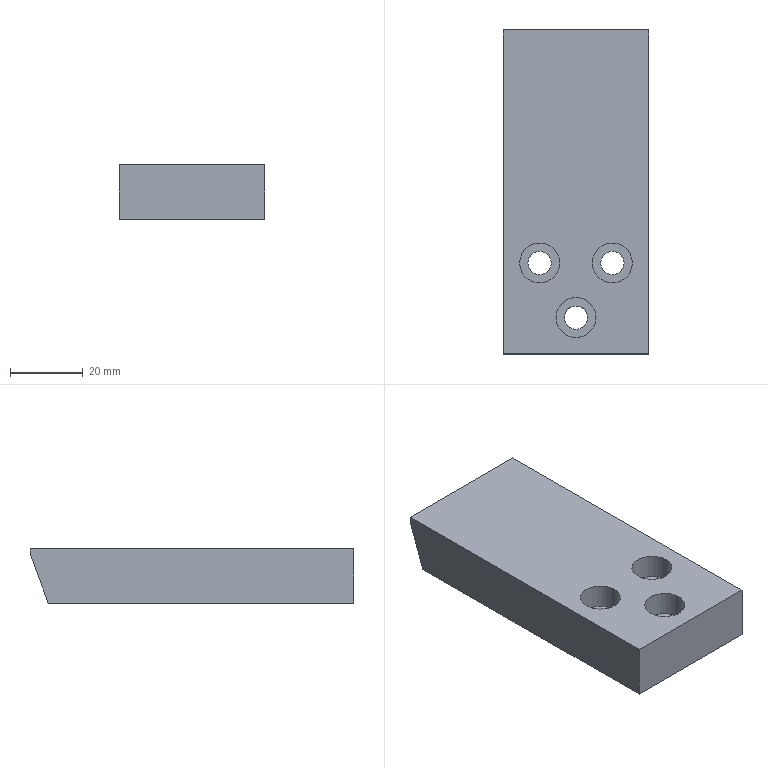Part | SolidWorks | features BaseBody 1 | 1 solid | 22 faces | box 40 x 89 x 15 mm | volume 49296 mm3 | cylinder 12 | plane 10 | commonest cylinder face diameters 6.4 x6 11 x6
STEP:
#1=CARTESIAN_POINT('',(4.5,25.,8.2));
#2=VERTEX_POINT('',#1);
#3=CARTESIAN_POINT('',(15.5,25.,8.2));
#4=VERTEX_POINT('',#3);
#5=CARTESIAN_POINT('',(10.,25.,8.2));
#6=DIRECTION('',(0.,0.,1.));
#7=DIRECTION('',(1.,0.,0.));
#8=AXIS2_PLACEMENT_3D('',#5,#6,#7);
#9=CIRCLE('',#8,5.5);
#10=EDGE_CURVE('',#2,#4,#9,.T.);
#11=ORIENTED_EDGE('',*,*,#10,.F.);
#12=CARTESIAN_POINT('',(4.5,25.,15.));
#13=VERTEX_POINT('',#12);
#14=CARTESIAN_POINT('',(4.5,25.,15.));
#15=DIRECTION('',(0.,0.,1.));
#16=VECTOR('',#15,1000.);
#17=LINE('',#14,#16);
#18=EDGE_CURVE('',#2,#13,#17,.T.);
#19=ORIENTED_EDGE('',*,*,#18,.T.);
#20=CARTESIAN_POINT('',(15.5,25.,15.));
#21=VERTEX_POINT('',#20);
#22=CARTESIAN_POINT('',(10.,25.,15.));
#23=DIRECTION('',(0.,0.,1.));
#24=DIRECTION('',(1.,0.,0.));
#25=AXIS2_PLACEMENT_3D('',#22,#23,#24);
#26=CIRCLE('',#25,5.5);
#27=EDGE_CURVE('',#13,#21,#26,.T.);
#28=ORIENTED_EDGE('',*,*,#27,.T.);
#29=CARTESIAN_POINT('',(15.5,25.,15.));
#30=DIRECTION('',(0.,0.,1.));
#31=VECTOR('',#30,1000.);
#32=LINE('',#29,#31);
#33=EDGE_CURVE('',#4,#21,#32,.T.);
#34=ORIENTED_EDGE('',*,*,#33,.F.);
#35=EDGE_LOOP('',(#11,#19,#28,#34));
#36=FACE_OUTER_BOUND('',#35,.T.);
#37=CARTESIAN_POINT('',(10.,25.,15.));
#38=DIRECTION('',(0.,0.,1.));
#39=DIRECTION('',(1.,0.,0.));
#40=AXIS2_PLACEMENT_3D('',#37,#38,#39);
#41=CYLINDRICAL_SURFACE('',#40,5.5);
#42=ADVANCED_FACE('',(#36),#41,.F.);
#43=CARTESIAN_POINT('',(6.8,25.,0.));
#44=VERTEX_POINT('',#43);
#45=CARTESIAN_POINT('',(13.2,25.,0.));
#46=VERTEX_POINT('',#45);
#47=CARTESIAN_POINT('',(10.,25.,0.));
#48=DIRECTION('',(0.,0.,1.));
#49=DIRECTION('',(1.,0.,0.));
#50=AXIS2_PLACEMENT_3D('',#47,#48,#49);
#51=CIRCLE('',#50,3.2);
#52=EDGE_CURVE('',#44,#46,#51,.T.);
#53=ORIENTED_EDGE('',*,*,#52,.F.);
#54=CARTESIAN_POINT('',(6.8,25.,8.2));
#55=VERTEX_POINT('',#54);
#56=CARTESIAN_POINT('',(6.8,25.,15.));
#57=DIRECTION('',(0.,0.,1.));
#58=VECTOR('',#57,1000.);
#59=LINE('',#56,#58);
#60=EDGE_CURVE('',#44,#55,#59,.T.);
#61=ORIENTED_EDGE('',*,*,#60,.T.);
#62=CARTESIAN_POINT('',(13.2,25.,8.2));
#63=VERTEX_POINT('',#62);
#64=CARTESIAN_POINT('',(10.,25.,8.2));
#65=DIRECTION('',(0.,0.,1.));
#66=DIRECTION('',(1.,0.,0.));
#67=AXIS2_PLACEMENT_3D('',#64,#65,#66);
#68=CIRCLE('',#67,3.2);
#69=EDGE_CURVE('',#55,#63,#68,.T.);
#70=ORIENTED_EDGE('',*,*,#69,.T.);
#71=CARTESIAN_POINT('',(13.2,25.,15.));
#72=DIRECTION('',(0.,0.,1.));
#73=VECTOR('',#72,1000.);
#74=LINE('',#71,#73);
#75=EDGE_CURVE('',#46,#63,#74,.T.);
#76=ORIENTED_EDGE('',*,*,#75,.F.);
#77=EDGE_LOOP('',(#53,#61,#70,#76));
#78=FACE_OUTER_BOUND('',#77,.T.);
#79=CARTESIAN_POINT('',(10.,25.,15.));
#80=DIRECTION('',(0.,0.,1.));
#81=DIRECTION('',(1.,0.,0.));
#82=AXIS2_PLACEMENT_3D('',#79,#80,#81);
#83=CYLINDRICAL_SURFACE('',#82,3.2);
#84=ADVANCED_FACE('',(#78),#83,.F.);
#85=CARTESIAN_POINT('',(24.5,25.,8.2));
#86=VERTEX_POINT('',#85);
#87=CARTESIAN_POINT('',(35.5,25.,8.2));
#88=VERTEX_POINT('',#87);
#89=CARTESIAN_POINT('',(30.,25.,8.2));
#90=DIRECTION('',(0.,0.,1.));
#91=DIRECTION('',(1.,0.,0.));
#92=AXIS2_PLACEMENT_3D('',#89,#90,#91);
#93=CIRCLE('',#92,5.5);
#94=EDGE_CURVE('',#86,#88,#93,.T.);
#95=ORIENTED_EDGE('',*,*,#94,.F.);
#96=CARTESIAN_POINT('',(24.5,25.,15.));
#97=VERTEX_POINT('',#96);
#98=CARTESIAN_POINT('',(24.5,25.,15.));
#99=DIRECTION('',(0.,0.,1.));
#100=VECTOR('',#99,1000.);
#101=LINE('',#98,#100);
#102=EDGE_CURVE('',#86,#97,#101,.T.);
#103=ORIENTED_EDGE('',*,*,#102,.T.);
#104=CARTESIAN_POINT('',(35.5,25.,15.));
#105=VERTEX_POINT('',#104);
#106=CARTESIAN_POINT('',(30.,25.,15.));
#107=DIRECTION('',(0.,0.,1.));
#108=DIRECTION('',(1.,0.,0.));
#109=AXIS2_PLACEMENT_3D('',#106,#107,#108);
#110=CIRCLE('',#109,5.5);
#111=EDGE_CURVE('',#97,#105,#110,.T.);
#112=ORIENTED_EDGE('',*,*,#111,.T.);
#113=CARTESIAN_POINT('',(35.5,25.,15.));
#114=DIRECTION('',(0.,0.,1.));
#115=VECTOR('',#114,1000.);
#116=LINE('',#113,#115);
#117=EDGE_CURVE('',#88,#105,#116,.T.);
#118=ORIENTED_EDGE('',*,*,#117,.F.);
#119=EDGE_LOOP('',(#95,#103,#112,#118));
#120=FACE_OUTER_BOUND('',#119,.T.);
#121=CARTESIAN_POINT('',(30.,25.,15.));
#122=DIRECTION('',(0.,0.,1.));
#123=DIRECTION('',(1.,0.,0.));
#124=AXIS2_PLACEMENT_3D('',#121,#122,#123);
#125=CYLINDRICAL_SURFACE('',#124,5.5);
#126=ADVANCED_FACE('',(#120),#125,.F.);
#127=CARTESIAN_POINT('',(26.8,25.,0.));
#128=VERTEX_POINT('',#127);
#129=CARTESIAN_POINT('',(33.2,25.,0.));
#130=VERTEX_POINT('',#129);
#131=CARTESIAN_POINT('',(30.,25.,0.));
#132=DIRECTION('',(0.,0.,1.));
#133=DIRECTION('',(1.,0.,0.));
#134=AXIS2_PLACEMENT_3D('',#131,#132,#133);
#135=CIRCLE('',#134,3.2);
#136=EDGE_CURVE('',#128,#130,#135,.T.);
#137=ORIENTED_EDGE('',*,*,#136,.F.);
#138=CARTESIAN_POINT('',(26.8,25.,8.2));
#139=VERTEX_POINT('',#138);
#140=CARTESIAN_POINT('',(26.8,25.,15.));
#141=DIRECTION('',(0.,0.,1.));
#142=VECTOR('',#141,1000.);
#143=LINE('',#140,#142);
#144=EDGE_CURVE('',#128,#139,#143,.T.);
#145=ORIENTED_EDGE('',*,*,#144,.T.);
#146=CARTESIAN_POINT('',(33.2,25.,8.2));
#147=VERTEX_POINT('',#146);
#148=CARTESIAN_POINT('',(30.,25.,8.2));
#149=DIRECTION('',(0.,0.,1.));
#150=DIRECTION('',(1.,0.,0.));
#151=AXIS2_PLACEMENT_3D('',#148,#149,#150);
#152=CIRCLE('',#151,3.2);
#153=EDGE_CURVE('',#139,#147,#152,.T.);
#154=ORIENTED_EDGE('',*,*,#153,.T.);
#155=CARTESIAN_POINT('',(33.2,25.,15.));
#156=DIRECTION('',(0.,0.,1.));
#157=VECTOR('',#156,1000.);
#158=LINE('',#155,#157);
#159=EDGE_CURVE('',#130,#147,#158,.T.);
#160=ORIENTED_EDGE('',*,*,#159,.F.);
#161=EDGE_LOOP('',(#137,#145,#154,#160));
#162=FACE_OUTER_BOUND('',#161,.T.);
#163=CARTESIAN_POINT('',(30.,25.,15.));
#164=DIRECTION('',(0.,0.,1.));
#165=DIRECTION('',(1.,0.,0.));
#166=AXIS2_PLACEMENT_3D('',#163,#164,#165);
#167=CYLINDRICAL_SURFACE('',#166,3.2);
#168=ADVANCED_FACE('',(#162),#167,.F.);
#169=CARTESIAN_POINT('',(14.5,10.,8.2));
#170=VERTEX_POINT('',#169);
#171=CARTESIAN_POINT('',(25.5,10.,8.2));
#172=VERTEX_POINT('',#171);
#173=CARTESIAN_POINT('',(20.,10.,8.2));
#174=DIRECTION('',(0.,0.,1.));
#175=DIRECTION('',(1.,0.,0.));
#176=AXIS2_PLACEMENT_3D('',#173,#174,#175);
#177=CIRCLE('',#176,5.5);
#178=EDGE_CURVE('',#170,#172,#177,.T.);
#179=ORIENTED_EDGE('',*,*,#178,.F.);
#180=CARTESIAN_POINT('',(14.5,10.,15.));
#181=VERTEX_POINT('',#180);
#182=CARTESIAN_POINT('',(14.5,10.,15.));
#183=DIRECTION('',(0.,0.,1.));
#184=VECTOR('',#183,1000.);
#185=LINE('',#182,#184);
#186=EDGE_CURVE('',#170,#181,#185,.T.);
#187=ORIENTED_EDGE('',*,*,#186,.T.);
#188=CARTESIAN_POINT('',(25.5,10.,15.));
#189=VERTEX_POINT('',#188);
#190=CARTESIAN_POINT('',(20.,10.,15.));
#191=DIRECTION('',(0.,0.,1.));
#192=DIRECTION('',(1.,0.,0.));
#193=AXIS2_PLACEMENT_3D('',#190,#191,#192);
#194=CIRCLE('',#193,5.5);
#195=EDGE_CURVE('',#181,#189,#194,.T.);
#196=ORIENTED_EDGE('',*,*,#195,.T.);
#197=CARTESIAN_POINT('',(25.5,10.,15.));
#198=DIRECTION('',(0.,0.,1.));
#199=VECTOR('',#198,1000.);
#200=LINE('',#197,#199);
#201=EDGE_CURVE('',#172,#189,#200,.T.);
#202=ORIENTED_EDGE('',*,*,#201,.F.);
#203=EDGE_LOOP('',(#179,#187,#196,#202));
#204=FACE_OUTER_BOUND('',#203,.T.);
#205=CARTESIAN_POINT('',(20.,10.,15.));
#206=DIRECTION('',(0.,0.,1.));
#207=DIRECTION('',(1.,0.,0.));
#208=AXIS2_PLACEMENT_3D('',#205,#206,#207);
#209=CYLINDRICAL_SURFACE('',#208,5.5);
#210=ADVANCED_FACE('',(#204),#209,.F.);
#211=CARTESIAN_POINT('',(16.8,10.,0.));
#212=VERTEX_POINT('',#211);
#213=CARTESIAN_POINT('',(23.2,10.,0.));
#214=VERTEX_POINT('',#213);
#215=CARTESIAN_POINT('',(20.,10.,0.));
#216=DIRECTION('',(0.,0.,1.));
#217=DIRECTION('',(1.,0.,0.));
#218=AXIS2_PLACEMENT_3D('',#215,#216,#217);
#219=CIRCLE('',#218,3.2);
#220=EDGE_CURVE('',#212,#214,#219,.T.);
#221=ORIENTED_EDGE('',*,*,#220,.F.);
#222=CARTESIAN_POINT('',(16.8,10.,8.2));
#223=VERTEX_POINT('',#222);
#224=CARTESIAN_POINT('',(16.8,10.,15.));
#225=DIRECTION('',(0.,0.,1.));
#226=VECTOR('',#225,1000.);
#227=LINE('',#224,#226);
#228=EDGE_CURVE('',#212,#223,#227,.T.);
#229=ORIENTED_EDGE('',*,*,#228,.T.);
#230=CARTESIAN_POINT('',(23.2,10.,8.2));
#231=VERTEX_POINT('',#230);
#232=CARTESIAN_POINT('',(20.,10.,8.2));
#233=DIRECTION('',(0.,0.,1.));
#234=DIRECTION('',(1.,0.,0.));
#235=AXIS2_PLACEMENT_3D('',#232,#233,#234);
#236=CIRCLE('',#235,3.2);
#237=EDGE_CURVE('',#223,#231,#236,.T.);
#238=ORIENTED_EDGE('',*,*,#237,.T.);
#239=CARTESIAN_POINT('',(23.2,10.,15.));
#240=DIRECTION('',(0.,0.,1.));
#241=VECTOR('',#240,1000.);
#242=LINE('',#239,#241);
#243=EDGE_CURVE('',#214,#231,#242,.T.);
#244=ORIENTED_EDGE('',*,*,#243,.F.);
#245=EDGE_LOOP('',(#221,#229,#238,#244));
#246=FACE_OUTER_BOUND('',#245,.T.);
#247=CARTESIAN_POINT('',(20.,10.,15.));
#248=DIRECTION('',(0.,0.,1.));
#249=DIRECTION('',(1.,0.,0.));
#250=AXIS2_PLACEMENT_3D('',#247,#248,#249);
#251=CYLINDRICAL_SURFACE('',#250,3.2);
#252=ADVANCED_FACE('',(#246),#251,.F.);
#253=CARTESIAN_POINT('',(40.,84.,0.));
#254=VERTEX_POINT('',#253);
#255=CARTESIAN_POINT('',(40.,89.,13.737));
#256=VERTEX_POINT('',#255);
#257=CARTESIAN_POINT('',(40.,89.,13.737));
#258=DIRECTION('',(0.,0.342,0.9397));
#259=VECTOR('',#258,1000.);
#260=LINE('',#257,#259);
#261=EDGE_CURVE('',#254,#256,#260,.T.);
#262=ORIENTED_EDGE('',*,*,#261,.F.);
#263=CARTESIAN_POINT('',(0.,84.,0.));
#264=VERTEX_POINT('',#263);
#265=CARTESIAN_POINT('',(40.,84.,0.));
#266=DIRECTION('',(1.,0.,0.));
#267=VECTOR('',#266,1000.);
#268=LINE('',#265,#267);
#269=EDGE_CURVE('',#264,#254,#268,.T.);
#270=ORIENTED_EDGE('',*,*,#269,.F.);
#271=CARTESIAN_POINT('',(0.,89.,13.737));
#272=VERTEX_POINT('',#271);
#273=CARTESIAN_POINT('',(0.,89.,13.737));
#274=DIRECTION('',(0.,-0.342,-0.9397));
#275=VECTOR('',#274,1000.);
#276=LINE('',#273,#275);
#277=EDGE_CURVE('',#272,#264,#276,.T.);
#278=ORIENTED_EDGE('',*,*,#277,.F.);
#279=CARTESIAN_POINT('',(0.,89.,13.737));
#280=DIRECTION('',(-1.,0.,0.));
#281=VECTOR('',#280,1000.);
#282=LINE('',#279,#281);
#283=EDGE_CURVE('',#256,#272,#282,.T.);
#284=ORIENTED_EDGE('',*,*,#283,.F.);
#285=EDGE_LOOP('',(#262,#270,#278,#284));
#286=FACE_OUTER_BOUND('',#285,.T.);
#287=CARTESIAN_POINT('',(0.,89.,13.737));
#288=DIRECTION('',(0.,0.9397,-0.342));
#289=DIRECTION('',(-1.,0.,0.));
#290=AXIS2_PLACEMENT_3D('',#287,#288,#289);
#291=PLANE('',#290);
#292=ADVANCED_FACE('',(#286),#291,.T.);
#293=CARTESIAN_POINT('',(10.,25.,8.2));
#294=DIRECTION('',(0.,0.,1.));
#295=DIRECTION('',(1.,0.,0.));
#296=AXIS2_PLACEMENT_3D('',#293,#294,#295);
#297=CIRCLE('',#296,3.2);
#298=EDGE_CURVE('',#63,#55,#297,.T.);
#299=ORIENTED_EDGE('',*,*,#298,.F.);
#300=ORIENTED_EDGE('',*,*,#69,.F.);
#301=EDGE_LOOP('',(#299,#300));
#302=FACE_BOUND('',#301,.T.);
#303=CARTESIAN_POINT('',(10.,25.,8.2));
#304=DIRECTION('',(0.,0.,1.));
#305=DIRECTION('',(1.,0.,0.));
#306=AXIS2_PLACEMENT_3D('',#303,#304,#305);
#307=CIRCLE('',#306,5.5);
#308=EDGE_CURVE('',#4,#2,#307,.T.);
#309=ORIENTED_EDGE('',*,*,#308,.T.);
#310=ORIENTED_EDGE('',*,*,#10,.T.);
#311=EDGE_LOOP('',(#309,#310));
#312=FACE_OUTER_BOUND('',#311,.T.);
#313=CARTESIAN_POINT('',(13.2,25.,8.2));
#314=DIRECTION('',(0.,0.,-1.));
#315=DIRECTION('',(0.,-1.,0.));
#316=AXIS2_PLACEMENT_3D('',#313,#314,#315);
#317=PLANE('',#316);
#318=ADVANCED_FACE('',(#302,#312),#317,.F.);
#319=CARTESIAN_POINT('',(30.,25.,8.2));
#320=DIRECTION('',(0.,0.,1.));
#321=DIRECTION('',(1.,0.,0.));
#322=AXIS2_PLACEMENT_3D('',#319,#320,#321);
#323=CIRCLE('',#322,3.2);
#324=EDGE_CURVE('',#147,#139,#323,.T.);
#325=ORIENTED_EDGE('',*,*,#324,.F.);
#326=ORIENTED_EDGE('',*,*,#153,.F.);
#327=EDGE_LOOP('',(#325,#326));
#328=FACE_BOUND('',#327,.T.);
#329=CARTESIAN_POINT('',(30.,25.,8.2));
#330=DIRECTION('',(0.,0.,1.));
#331=DIRECTION('',(1.,0.,0.));
#332=AXIS2_PLACEMENT_3D('',#329,#330,#331);
#333=CIRCLE('',#332,5.5);
#334=EDGE_CURVE('',#88,#86,#333,.T.);
#335=ORIENTED_EDGE('',*,*,#334,.T.);
#336=ORIENTED_EDGE('',*,*,#94,.T.);
#337=EDGE_LOOP('',(#335,#336));
#338=FACE_OUTER_BOUND('',#337,.T.);
#339=CARTESIAN_POINT('',(33.2,25.,8.2));
#340=DIRECTION('',(0.,0.,-1.));
#341=DIRECTION('',(0.,-1.,0.));
#342=AXIS2_PLACEMENT_3D('',#339,#340,#341);
#343=PLANE('',#342);
#344=ADVANCED_FACE('',(#328,#338),#343,.F.);
#345=CARTESIAN_POINT('',(20.,10.,8.2));
#346=DIRECTION('',(0.,0.,1.));
#347=DIRECTION('',(1.,0.,0.));
#348=AXIS2_PLACEMENT_3D('',#345,#346,#347);
#349=CIRCLE('',#348,3.2);
#350=EDGE_CURVE('',#231,#223,#349,.T.);
#351=ORIENTED_EDGE('',*,*,#350,.F.);
#352=ORIENTED_EDGE('',*,*,#237,.F.);
#353=EDGE_LOOP('',(#351,#352));
#354=FACE_BOUND('',#353,.T.);
#355=CARTESIAN_POINT('',(20.,10.,8.2));
#356=DIRECTION('',(0.,0.,1.));
#357=DIRECTION('',(1.,0.,0.));
#358=AXIS2_PLACEMENT_3D('',#355,#356,#357);
#359=CIRCLE('',#358,5.5);
#360=EDGE_CURVE('',#172,#170,#359,.T.);
#361=ORIENTED_EDGE('',*,*,#360,.T.);
#362=ORIENTED_EDGE('',*,*,#178,.T.);
#363=EDGE_LOOP('',(#361,#362));
#364=FACE_OUTER_BOUND('',#363,.T.);
#365=CARTESIAN_POINT('',(23.2,10.,8.2));
#366=DIRECTION('',(0.,0.,-1.));
#367=DIRECTION('',(0.,-1.,0.));
#368=AXIS2_PLACEMENT_3D('',#365,#366,#367);
#369=PLANE('',#368);
#370=ADVANCED_FACE('',(#354,#364),#369,.F.);
#371=CARTESIAN_POINT('',(20.,10.,0.));
#372=DIRECTION('',(0.,0.,1.));
#373=DIRECTION('',(1.,0.,0.));
#374=AXIS2_PLACEMENT_3D('',#371,#372,#373);
#375=CIRCLE('',#374,3.2);
#376=EDGE_CURVE('',#214,#212,#375,.T.);
#377=ORIENTED_EDGE('',*,*,#376,.T.);
#378=ORIENTED_EDGE('',*,*,#220,.T.);
#379=EDGE_LOOP('',(#377,#378));
#380=FACE_BOUND('',#379,.T.);
#381=CARTESIAN_POINT('',(30.,25.,0.));
#382=DIRECTION('',(0.,0.,1.));
#383=DIRECTION('',(1.,0.,0.));
#384=AXIS2_PLACEMENT_3D('',#381,#382,#383);
#385=CIRCLE('',#384,3.2);
#386=EDGE_CURVE('',#130,#128,#385,.T.);
#387=ORIENTED_EDGE('',*,*,#386,.T.);
#388=ORIENTED_EDGE('',*,*,#136,.T.);
#389=EDGE_LOOP('',(#387,#388));
#390=FACE_BOUND('',#389,.T.);
#391=CARTESIAN_POINT('',(10.,25.,0.));
#392=DIRECTION('',(0.,0.,1.));
#393=DIRECTION('',(1.,0.,0.));
#394=AXIS2_PLACEMENT_3D('',#391,#392,#393);
#395=CIRCLE('',#394,3.2);
#396=EDGE_CURVE('',#46,#44,#395,.T.);
#397=ORIENTED_EDGE('',*,*,#396,.T.);
#398=ORIENTED_EDGE('',*,*,#52,.T.);
#399=EDGE_LOOP('',(#397,#398));
#400=FACE_BOUND('',#399,.T.);
#401=CARTESIAN_POINT('',(0.,0.,0.));
#402=VERTEX_POINT('',#401);
#403=CARTESIAN_POINT('',(0.,0.,0.));
#404=DIRECTION('',(0.,-1.,0.));
#405=VECTOR('',#404,1000.);
#406=LINE('',#403,#405);
#407=EDGE_CURVE('',#264,#402,#406,.T.);
#408=ORIENTED_EDGE('',*,*,#407,.F.);
#409=ORIENTED_EDGE('',*,*,#269,.T.);
#410=CARTESIAN_POINT('',(40.,0.,0.));
#411=VERTEX_POINT('',#410);
#412=CARTESIAN_POINT('',(40.,0.,0.));
#413=DIRECTION('',(0.,1.,0.));
#414=VECTOR('',#413,1000.);
#415=LINE('',#412,#414);
#416=EDGE_CURVE('',#411,#254,#415,.T.);
#417=ORIENTED_EDGE('',*,*,#416,.F.);
#418=CARTESIAN_POINT('',(0.,0.,0.));
#419=DIRECTION('',(1.,0.,0.));
#420=VECTOR('',#419,1000.);
#421=LINE('',#418,#420);
#422=EDGE_CURVE('',#402,#411,#421,.T.);
#423=ORIENTED_EDGE('',*,*,#422,.F.);
#424=EDGE_LOOP('',(#408,#409,#417,#423));
#425=FACE_OUTER_BOUND('',#424,.T.);
#426=CARTESIAN_POINT('',(0.,0.,0.));
#427=DIRECTION('',(0.,0.,-1.));
#428=DIRECTION('',(0.,-1.,0.));
#429=AXIS2_PLACEMENT_3D('',#426,#427,#428);
#430=PLANE('',#429);
#431=ADVANCED_FACE('',(#380,#390,#400,#425),#430,.T.);
#432=CARTESIAN_POINT('',(20.,10.,15.));
#433=DIRECTION('',(0.,0.,1.));
#434=DIRECTION('',(1.,0.,0.));
#435=AXIS2_PLACEMENT_3D('',#432,#433,#434);
#436=CIRCLE('',#435,5.5);
#437=EDGE_CURVE('',#189,#181,#436,.T.);
#438=ORIENTED_EDGE('',*,*,#437,.F.);
#439=ORIENTED_EDGE('',*,*,#195,.F.);
#440=EDGE_LOOP('',(#438,#439));
#441=FACE_BOUND('',#440,.T.);
#442=CARTESIAN_POINT('',(30.,25.,15.));
#443=DIRECTION('',(0.,0.,1.));
#444=DIRECTION('',(1.,0.,0.));
#445=AXIS2_PLACEMENT_3D('',#442,#443,#444);
#446=CIRCLE('',#445,5.5);
#447=EDGE_CURVE('',#105,#97,#446,.T.);
#448=ORIENTED_EDGE('',*,*,#447,.F.);
#449=ORIENTED_EDGE('',*,*,#111,.F.);
#450=EDGE_LOOP('',(#448,#449));
#451=FACE_BOUND('',#450,.T.);
#452=CARTESIAN_POINT('',(10.,25.,15.));
#453=DIRECTION('',(0.,0.,1.));
#454=DIRECTION('',(1.,0.,0.));
#455=AXIS2_PLACEMENT_3D('',#452,#453,#454);
#456=CIRCLE('',#455,5.5);
#457=EDGE_CURVE('',#21,#13,#456,.T.);
#458=ORIENTED_EDGE('',*,*,#457,.F.);
#459=ORIENTED_EDGE('',*,*,#27,.F.);
#460=EDGE_LOOP('',(#458,#459));
#461=FACE_BOUND('',#460,.T.);
#462=CARTESIAN_POINT('',(0.,89.,15.));
#463=VERTEX_POINT('',#462);
#464=CARTESIAN_POINT('',(0.,0.,15.));
#465=VERTEX_POINT('',#464);
#466=CARTESIAN_POINT('',(0.,0.,15.));
#467=DIRECTION('',(0.,-1.,0.));
#468=VECTOR('',#467,1000.);
#469=LINE('',#466,#468);
#470=EDGE_CURVE('',#463,#465,#469,.T.);
#471=ORIENTED_EDGE('',*,*,#470,.T.);
#472=CARTESIAN_POINT('',(40.,0.,15.));
#473=VERTEX_POINT('',#472);
#474=CARTESIAN_POINT('',(0.,0.,15.));
#475=DIRECTION('',(1.,0.,0.));
#476=VECTOR('',#475,1000.);
#477=LINE('',#474,#476);
#478=EDGE_CURVE('',#465,#473,#477,.T.);
#479=ORIENTED_EDGE('',*,*,#478,.T.);
#480=CARTESIAN_POINT('',(40.,89.,15.));
#481=VERTEX_POINT('',#480);
#482=CARTESIAN_POINT('',(40.,0.,15.));
#483=DIRECTION('',(0.,1.,0.));
#484=VECTOR('',#483,1000.);
#485=LINE('',#482,#484);
#486=EDGE_CURVE('',#473,#481,#485,.T.);
#487=ORIENTED_EDGE('',*,*,#486,.T.);
#488=CARTESIAN_POINT('',(0.,89.,15.));
#489=DIRECTION('',(-1.,0.,0.));
#490=VECTOR('',#489,1000.);
#491=LINE('',#488,#490);
#492=EDGE_CURVE('',#481,#463,#491,.T.);
#493=ORIENTED_EDGE('',*,*,#492,.T.);
#494=EDGE_LOOP('',(#471,#479,#487,#493));
#495=FACE_OUTER_BOUND('',#494,.T.);
#496=CARTESIAN_POINT('',(0.,0.,15.));
#497=DIRECTION('',(0.,0.,-1.));
#498=DIRECTION('',(0.,-1.,0.));
#499=AXIS2_PLACEMENT_3D('',#496,#497,#498);
#500=PLANE('',#499);
#501=ADVANCED_FACE('',(#441,#451,#461,#495),#500,.F.);
#502=CARTESIAN_POINT('',(40.,89.,15.));
#503=DIRECTION('',(0.,0.,-1.));
#504=VECTOR('',#503,1000.);
#505=LINE('',#502,#504);
#506=EDGE_CURVE('',#481,#256,#505,.T.);
#507=ORIENTED_EDGE('',*,*,#506,.T.);
#508=ORIENTED_EDGE('',*,*,#283,.T.);
#509=CARTESIAN_POINT('',(0.,89.,15.));
#510=DIRECTION('',(0.,0.,-1.));
#511=VECTOR('',#510,1000.);
#512=LINE('',#509,#511);
#513=EDGE_CURVE('',#463,#272,#512,.T.);
#514=ORIENTED_EDGE('',*,*,#513,.F.);
#515=ORIENTED_EDGE('',*,*,#492,.F.);
#516=EDGE_LOOP('',(#507,#508,#514,#515));
#517=FACE_OUTER_BOUND('',#516,.T.);
#518=CARTESIAN_POINT('',(0.,89.,15.));
#519=DIRECTION('',(0.,-1.,0.));
#520=DIRECTION('',(0.,0.,-1.));
#521=AXIS2_PLACEMENT_3D('',#518,#519,#520);
#522=PLANE('',#521);
#523=ADVANCED_FACE('',(#517),#522,.F.);
#524=ORIENTED_EDGE('',*,*,#416,.T.);
#525=ORIENTED_EDGE('',*,*,#261,.T.);
#526=ORIENTED_EDGE('',*,*,#506,.F.);
#527=ORIENTED_EDGE('',*,*,#486,.F.);
#528=CARTESIAN_POINT('',(40.,0.,15.));
#529=DIRECTION('',(0.,0.,-1.));
#530=VECTOR('',#529,1000.);
#531=LINE('',#528,#530);
#532=EDGE_CURVE('',#473,#411,#531,.T.);
#533=ORIENTED_EDGE('',*,*,#532,.T.);
#534=EDGE_LOOP('',(#524,#525,#526,#527,#533));
#535=FACE_OUTER_BOUND('',#534,.T.);
#536=CARTESIAN_POINT('',(40.,0.,15.));
#537=DIRECTION('',(-1.,0.,0.));
#538=DIRECTION('',(0.,0.,1.));
#539=AXIS2_PLACEMENT_3D('',#536,#537,#538);
#540=PLANE('',#539);
#541=ADVANCED_FACE('',(#535),#540,.F.);
#542=ORIENTED_EDGE('',*,*,#422,.T.);
#543=ORIENTED_EDGE('',*,*,#532,.F.);
#544=ORIENTED_EDGE('',*,*,#478,.F.);
#545=CARTESIAN_POINT('',(0.,0.,15.));
#546=DIRECTION('',(0.,0.,-1.));
#547=VECTOR('',#546,1000.);
#548=LINE('',#545,#547);
#549=EDGE_CURVE('',#465,#402,#548,.T.);
#550=ORIENTED_EDGE('',*,*,#549,.T.);
#551=EDGE_LOOP('',(#542,#543,#544,#550));
#552=FACE_OUTER_BOUND('',#551,.T.);
#553=CARTESIAN_POINT('',(0.,0.,15.));
#554=DIRECTION('',(0.,1.,0.));
#555=DIRECTION('',(1.,0.,0.));
#556=AXIS2_PLACEMENT_3D('',#553,#554,#555);
#557=PLANE('',#556);
#558=ADVANCED_FACE('',(#552),#557,.F.);
#559=ORIENTED_EDGE('',*,*,#513,.T.);
#560=ORIENTED_EDGE('',*,*,#277,.T.);
#561=ORIENTED_EDGE('',*,*,#407,.T.);
#562=ORIENTED_EDGE('',*,*,#549,.F.);
#563=ORIENTED_EDGE('',*,*,#470,.F.);
#564=EDGE_LOOP('',(#559,#560,#561,#562,#563));
#565=FACE_OUTER_BOUND('',#564,.T.);
#566=CARTESIAN_POINT('',(0.,0.,15.));
#567=DIRECTION('',(1.,0.,0.));
#568=DIRECTION('',(0.,1.,0.));
#569=AXIS2_PLACEMENT_3D('',#566,#567,#568);
#570=PLANE('',#569);
#571=ADVANCED_FACE('',(#565),#570,.F.);
#572=ORIENTED_EDGE('',*,*,#228,.F.);
#573=ORIENTED_EDGE('',*,*,#376,.F.);
#574=ORIENTED_EDGE('',*,*,#243,.T.);
#575=ORIENTED_EDGE('',*,*,#350,.T.);
#576=EDGE_LOOP('',(#572,#573,#574,#575));
#577=FACE_OUTER_BOUND('',#576,.T.);
#578=CARTESIAN_POINT('',(20.,10.,15.));
#579=DIRECTION('',(0.,0.,1.));
#580=DIRECTION('',(1.,0.,0.));
#581=AXIS2_PLACEMENT_3D('',#578,#579,#580);
#582=CYLINDRICAL_SURFACE('',#581,3.2);
#583=ADVANCED_FACE('',(#577),#582,.F.);
#584=ORIENTED_EDGE('',*,*,#186,.F.);
#585=ORIENTED_EDGE('',*,*,#360,.F.);
#586=ORIENTED_EDGE('',*,*,#201,.T.);
#587=ORIENTED_EDGE('',*,*,#437,.T.);
#588=EDGE_LOOP('',(#584,#585,#586,#587));
#589=FACE_OUTER_BOUND('',#588,.T.);
#590=CARTESIAN_POINT('',(20.,10.,15.));
#591=DIRECTION('',(0.,0.,1.));
#592=DIRECTION('',(1.,0.,0.));
#593=AXIS2_PLACEMENT_3D('',#590,#591,#592);
#594=CYLINDRICAL_SURFACE('',#593,5.5);
#595=ADVANCED_FACE('',(#589),#594,.F.);
#596=ORIENTED_EDGE('',*,*,#144,.F.);
#597=ORIENTED_EDGE('',*,*,#386,.F.);
#598=ORIENTED_EDGE('',*,*,#159,.T.);
#599=ORIENTED_EDGE('',*,*,#324,.T.);
#600=EDGE_LOOP('',(#596,#597,#598,#599));
#601=FACE_OUTER_BOUND('',#600,.T.);
#602=CARTESIAN_POINT('',(30.,25.,15.));
#603=DIRECTION('',(0.,0.,1.));
#604=DIRECTION('',(1.,0.,0.));
#605=AXIS2_PLACEMENT_3D('',#602,#603,#604);
#606=CYLINDRICAL_SURFACE('',#605,3.2);
#607=ADVANCED_FACE('',(#601),#606,.F.);
#608=ORIENTED_EDGE('',*,*,#102,.F.);
#609=ORIENTED_EDGE('',*,*,#334,.F.);
#610=ORIENTED_EDGE('',*,*,#117,.T.);
#611=ORIENTED_EDGE('',*,*,#447,.T.);
#612=EDGE_LOOP('',(#608,#609,#610,#611));
#613=FACE_OUTER_BOUND('',#612,.T.);
#614=CARTESIAN_POINT('',(30.,25.,15.));
#615=DIRECTION('',(0.,0.,1.));
#616=DIRECTION('',(1.,0.,0.));
#617=AXIS2_PLACEMENT_3D('',#614,#615,#616);
#618=CYLINDRICAL_SURFACE('',#617,5.5);
#619=ADVANCED_FACE('',(#613),#618,.F.);
#620=ORIENTED_EDGE('',*,*,#60,.F.);
#621=ORIENTED_EDGE('',*,*,#396,.F.);
#622=ORIENTED_EDGE('',*,*,#75,.T.);
#623=ORIENTED_EDGE('',*,*,#298,.T.);
#624=EDGE_LOOP('',(#620,#621,#622,#623));
#625=FACE_OUTER_BOUND('',#624,.T.);
#626=CARTESIAN_POINT('',(10.,25.,15.));
#627=DIRECTION('',(0.,0.,1.));
#628=DIRECTION('',(1.,0.,0.));
#629=AXIS2_PLACEMENT_3D('',#626,#627,#628);
#630=CYLINDRICAL_SURFACE('',#629,3.2);
#631=ADVANCED_FACE('',(#625),#630,.F.);
#632=ORIENTED_EDGE('',*,*,#18,.F.);
#633=ORIENTED_EDGE('',*,*,#308,.F.);
#634=ORIENTED_EDGE('',*,*,#33,.T.);
#635=ORIENTED_EDGE('',*,*,#457,.T.);
#636=EDGE_LOOP('',(#632,#633,#634,#635));
#637=FACE_OUTER_BOUND('',#636,.T.);
#638=CARTESIAN_POINT('',(10.,25.,15.));
#639=DIRECTION('',(0.,0.,1.));
#640=DIRECTION('',(1.,0.,0.));
#641=AXIS2_PLACEMENT_3D('',#638,#639,#640);
#642=CYLINDRICAL_SURFACE('',#641,5.5);
#643=ADVANCED_FACE('',(#637),#642,.F.);
#644=CLOSED_SHELL('',(#42,#84,#126,#168,#210,#252,#292,#318,#344,#370,#431,#501,#523,#541,#558,#571,#583,#595,#607,#619,#631,#643));
#645=MANIFOLD_SOLID_BREP('',#644);
#646=CARTESIAN_POINT('',(0.,0.,0.));
#647=DIRECTION('',(0.,0.,1.));
#648=DIRECTION('',(1.,0.,0.));
#649=AXIS2_PLACEMENT_3D('',#646,#647,#648);
#650=(LENGTH_UNIT()NAMED_UNIT(*)SI_UNIT(.MILLI.,.METRE.));
#651=UNCERTAINTY_MEASURE_WITH_UNIT(LENGTH_MEASURE(0.00001),#650,'','');
#652=(NAMED_UNIT(*)PLANE_ANGLE_UNIT()SI_UNIT($,.RADIAN.));
#653=(NAMED_UNIT(*)SI_UNIT($,.STERADIAN.)SOLID_ANGLE_UNIT());
#654=(GEOMETRIC_REPRESENTATION_CONTEXT(3)GLOBAL_UNCERTAINTY_ASSIGNED_CONTEXT((#651))GLOBAL_UNIT_ASSIGNED_CONTEXT((#650,#652,#653))REPRESENTATION_CONTEXT('',''));
#655=ADVANCED_BREP_SHAPE_REPRESENTATION('',(#645,#649),#654);